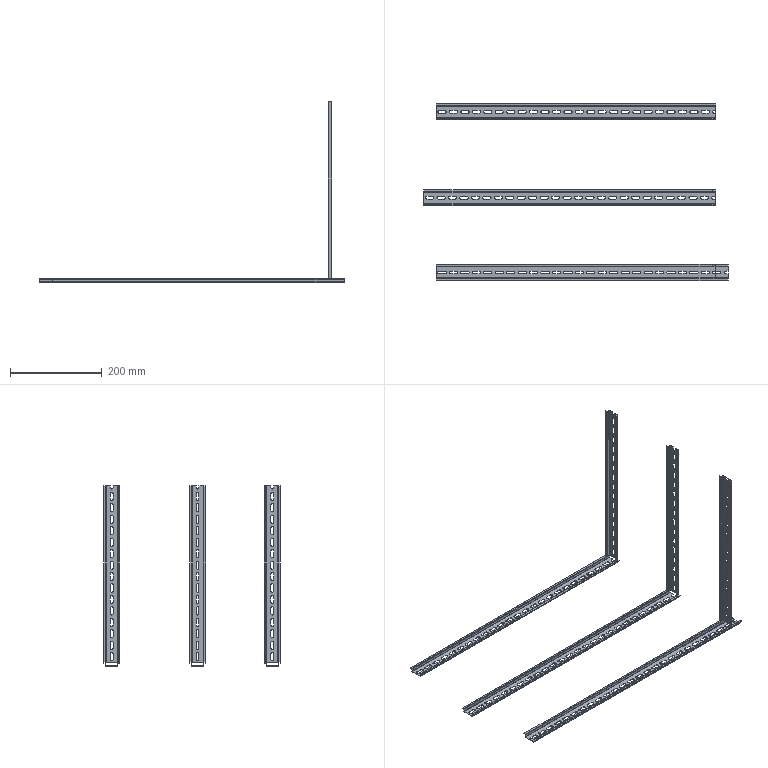Part | SolidWorks | 6 solids | 632 faces | box 664 x 385.75 x 394.5 mm | volume 131312 mm3 | plane 340 | cylinder 292 | commonest cylinder face diameters 6.3 x244 1 x24 2 x24